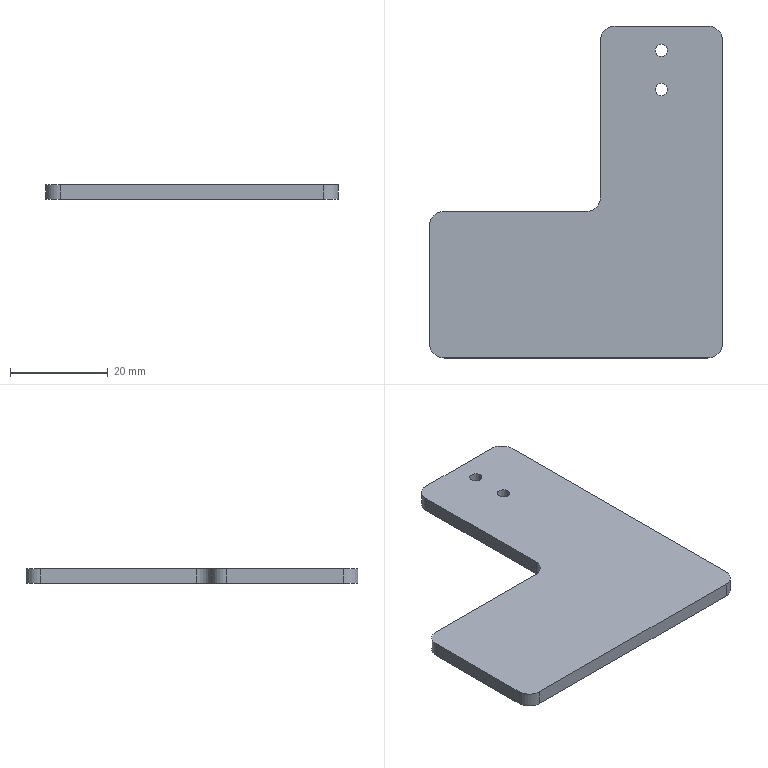Part | STEP file | 001-006-Pre-insertion mechanism drag chain mounting plate | 1 solid | 18 faces | box 60 x 68 x 3 mm | volume 8197 mm3 | cylinder 10 | plane 8 | commonest cylinder face diameters 6 x6 2.5 x4
STEP:
#1=CARTESIAN_POINT('',(0.,0.,0.));
#2=DIRECTION('',(0.,0.,1.));
#3=DIRECTION('',(1.,0.,0.));
#4=AXIS2_PLACEMENT_3D('',#1,#2,#3);
#5=CARTESIAN_POINT('',(18.75,29.,-3.));
#6=VERTEX_POINT('',#5);
#7=CARTESIAN_POINT('',(18.75,29.,0.));
#8=VERTEX_POINT('',#7);
#9=CARTESIAN_POINT('',(18.75,29.,0.));
#10=DIRECTION('',(0.,0.,1.));
#11=VECTOR('',#10,1.);
#12=LINE('',#9,#11);
#13=CARTESIAN_POINT('',(17.5,29.,0.));
#14=DIRECTION('',(0.,0.,1.));
#15=DIRECTION('',(1.,0.,0.));
#16=AXIS2_PLACEMENT_3D('',#13,#14,#15);
#17=CYLINDRICAL_SURFACE('',#16,1.25);
#18=CARTESIAN_POINT('',(6.283,0.));
#19=DIRECTION('',(0.,1.));
#20=VECTOR('',#19,1.);
#21=LINE('',#18,#20);
#22=(GEOMETRIC_REPRESENTATION_CONTEXT(2)PARAMETRIC_REPRESENTATION_CONTEXT()REPRESENTATION_CONTEXT('',''));
#23=DEFINITIONAL_REPRESENTATION('',(#21),#22);
#24=PCURVE('',#17,#23);
#25=CARTESIAN_POINT('',(17.5,29.,0.));
#26=DIRECTION('',(0.,0.,1.));
#27=DIRECTION('',(1.,0.,0.));
#28=AXIS2_PLACEMENT_3D('',#25,#26,#27);
#29=CYLINDRICAL_SURFACE('',#28,1.25);
#30=CARTESIAN_POINT('',(0.,0.));
#31=DIRECTION('',(0.,1.));
#32=VECTOR('',#31,1.);
#33=LINE('',#30,#32);
#34=(GEOMETRIC_REPRESENTATION_CONTEXT(2)PARAMETRIC_REPRESENTATION_CONTEXT()REPRESENTATION_CONTEXT('',''));
#35=DEFINITIONAL_REPRESENTATION('',(#33),#34);
#36=PCURVE('',#29,#35);
#37=SURFACE_CURVE('',#12,(#24,#36),.PCURVE_S1.);
#38=EDGE_CURVE('',#6,#8,#37,.T.);
#39=ORIENTED_EDGE('',*,*,#38,.T.);
#40=CARTESIAN_POINT('',(16.25,29.,0.));
#41=VERTEX_POINT('',#40);
#42=CARTESIAN_POINT('',(17.5,29.,0.));
#43=DIRECTION('',(0.,0.,1.));
#44=DIRECTION('',(1.,0.,0.));
#45=AXIS2_PLACEMENT_3D('',#42,#43,#44);
#46=CIRCLE('',#45,1.25);
#47=CARTESIAN_POINT('',(0.,0.));
#48=DIRECTION('',(1.,0.));
#49=VECTOR('',#48,1.);
#50=LINE('',#47,#49);
#51=(GEOMETRIC_REPRESENTATION_CONTEXT(2)PARAMETRIC_REPRESENTATION_CONTEXT()REPRESENTATION_CONTEXT('',''));
#52=DEFINITIONAL_REPRESENTATION('',(#50),#51);
#53=PCURVE('',#17,#52);
#54=CARTESIAN_POINT('',(0.,0.,0.));
#55=DIRECTION('',(0.,0.,-1.));
#56=DIRECTION('',(-1.,0.,0.));
#57=AXIS2_PLACEMENT_3D('',#54,#55,#56);
#58=PLANE('',#57);
#59=CARTESIAN_POINT('',(-18.75,29.));
#60=CARTESIAN_POINT('',(-18.75,31.165));
#61=CARTESIAN_POINT('',(-16.875,30.083));
#62=CARTESIAN_POINT('',(-15.,29.));
#63=CARTESIAN_POINT('',(-16.875,27.917));
#64=CARTESIAN_POINT('',(-18.75,26.835));
#65=CARTESIAN_POINT('',(-18.75,29.));
#66=(BOUNDED_CURVE()B_SPLINE_CURVE(2,(#59,#60,#61,#62,#63,#64,#65),.UNSPECIFIED.,.T.,.F.)B_SPLINE_CURVE_WITH_KNOTS((1,2,2,2,2,1),(-2.094,0.,2.094,4.189,6.283,8.378),.UNSPECIFIED.)CURVE()GEOMETRIC_REPRESENTATION_ITEM()RATIONAL_B_SPLINE_CURVE((1.,0.5,1.,0.5,1.,0.5,1.))REPRESENTATION_ITEM(''));
#67=(GEOMETRIC_REPRESENTATION_CONTEXT(2)PARAMETRIC_REPRESENTATION_CONTEXT()REPRESENTATION_CONTEXT('',''));
#68=DEFINITIONAL_REPRESENTATION('',(#66),#67);
#69=PCURVE('',#58,#68);
#70=SURFACE_CURVE('',#46,(#53,#69),.PCURVE_S1.);
#71=EDGE_CURVE('',#41,#8,#70,.T.);
#72=ORIENTED_EDGE('',*,*,#71,.F.);
#73=CARTESIAN_POINT('',(16.25,29.,-3.));
#74=VERTEX_POINT('',#73);
#75=CARTESIAN_POINT('',(16.25,29.,0.));
#76=DIRECTION('',(0.,0.,1.));
#77=VECTOR('',#76,1.);
#78=LINE('',#75,#77);
#79=CARTESIAN_POINT('',(3.142,0.));
#80=DIRECTION('',(0.,1.));
#81=VECTOR('',#80,1.);
#82=LINE('',#79,#81);
#83=(GEOMETRIC_REPRESENTATION_CONTEXT(2)PARAMETRIC_REPRESENTATION_CONTEXT()REPRESENTATION_CONTEXT('',''));
#84=DEFINITIONAL_REPRESENTATION('',(#82),#83);
#85=PCURVE('',#17,#84);
#86=CARTESIAN_POINT('',(3.142,0.));
#87=DIRECTION('',(0.,1.));
#88=VECTOR('',#87,1.);
#89=LINE('',#86,#88);
#90=(GEOMETRIC_REPRESENTATION_CONTEXT(2)PARAMETRIC_REPRESENTATION_CONTEXT()REPRESENTATION_CONTEXT('',''));
#91=DEFINITIONAL_REPRESENTATION('',(#89),#90);
#92=PCURVE('',#29,#91);
#93=SURFACE_CURVE('',#78,(#85,#92),.PCURVE_S1.);
#94=EDGE_CURVE('',#74,#41,#93,.T.);
#95=ORIENTED_EDGE('',*,*,#94,.F.);
#96=CARTESIAN_POINT('',(17.5,29.,-3.));
#97=DIRECTION('',(0.,0.,1.));
#98=DIRECTION('',(1.,0.,0.));
#99=AXIS2_PLACEMENT_3D('',#96,#97,#98);
#100=CIRCLE('',#99,1.25);
#101=CARTESIAN_POINT('',(0.,-3.));
#102=DIRECTION('',(1.,0.));
#103=VECTOR('',#102,1.);
#104=LINE('',#101,#103);
#105=(GEOMETRIC_REPRESENTATION_CONTEXT(2)PARAMETRIC_REPRESENTATION_CONTEXT()REPRESENTATION_CONTEXT('',''));
#106=DEFINITIONAL_REPRESENTATION('',(#104),#105);
#107=PCURVE('',#17,#106);
#108=CARTESIAN_POINT('',(0.,0.,-3.));
#109=DIRECTION('',(0.,0.,-1.));
#110=DIRECTION('',(-1.,0.,0.));
#111=AXIS2_PLACEMENT_3D('',#108,#109,#110);
#112=PLANE('',#111);
#113=CARTESIAN_POINT('',(-18.75,29.));
#114=CARTESIAN_POINT('',(-18.75,31.165));
#115=CARTESIAN_POINT('',(-16.875,30.083));
#116=CARTESIAN_POINT('',(-15.,29.));
#117=CARTESIAN_POINT('',(-16.875,27.917));
#118=CARTESIAN_POINT('',(-18.75,26.835));
#119=CARTESIAN_POINT('',(-18.75,29.));
#120=(BOUNDED_CURVE()B_SPLINE_CURVE(2,(#113,#114,#115,#116,#117,#118,#119),.UNSPECIFIED.,.T.,.F.)B_SPLINE_CURVE_WITH_KNOTS((1,2,2,2,2,1),(-2.094,0.,2.094,4.189,6.283,8.378),.UNSPECIFIED.)CURVE()GEOMETRIC_REPRESENTATION_ITEM()RATIONAL_B_SPLINE_CURVE((1.,0.5,1.,0.5,1.,0.5,1.))REPRESENTATION_ITEM(''));
#121=(GEOMETRIC_REPRESENTATION_CONTEXT(2)PARAMETRIC_REPRESENTATION_CONTEXT()REPRESENTATION_CONTEXT('',''));
#122=DEFINITIONAL_REPRESENTATION('',(#120),#121);
#123=PCURVE('',#112,#122);
#124=SURFACE_CURVE('',#100,(#107,#123),.PCURVE_S1.);
#125=EDGE_CURVE('',#74,#6,#124,.T.);
#126=ORIENTED_EDGE('',*,*,#125,.T.);
#127=EDGE_LOOP('',(#39,#72,#95,#126));
#128=FACE_BOUND('',#127,.F.);
#129=ADVANCED_FACE('',(#128),#17,.F.);
#130=CARTESIAN_POINT('',(18.75,21.,-3.));
#131=VERTEX_POINT('',#130);
#132=CARTESIAN_POINT('',(18.75,21.,0.));
#133=VERTEX_POINT('',#132);
#134=CARTESIAN_POINT('',(18.75,21.,0.));
#135=DIRECTION('',(0.,0.,1.));
#136=VECTOR('',#135,1.);
#137=LINE('',#134,#136);
#138=CARTESIAN_POINT('',(17.5,21.,0.));
#139=DIRECTION('',(0.,0.,1.));
#140=DIRECTION('',(1.,0.,0.));
#141=AXIS2_PLACEMENT_3D('',#138,#139,#140);
#142=CYLINDRICAL_SURFACE('',#141,1.25);
#143=CARTESIAN_POINT('',(6.283,0.));
#144=DIRECTION('',(0.,1.));
#145=VECTOR('',#144,1.);
#146=LINE('',#143,#145);
#147=(GEOMETRIC_REPRESENTATION_CONTEXT(2)PARAMETRIC_REPRESENTATION_CONTEXT()REPRESENTATION_CONTEXT('',''));
#148=DEFINITIONAL_REPRESENTATION('',(#146),#147);
#149=PCURVE('',#142,#148);
#150=CARTESIAN_POINT('',(17.5,21.,0.));
#151=DIRECTION('',(0.,0.,1.));
#152=DIRECTION('',(1.,0.,0.));
#153=AXIS2_PLACEMENT_3D('',#150,#151,#152);
#154=CYLINDRICAL_SURFACE('',#153,1.25);
#155=CARTESIAN_POINT('',(0.,0.));
#156=DIRECTION('',(0.,1.));
#157=VECTOR('',#156,1.);
#158=LINE('',#155,#157);
#159=(GEOMETRIC_REPRESENTATION_CONTEXT(2)PARAMETRIC_REPRESENTATION_CONTEXT()REPRESENTATION_CONTEXT('',''));
#160=DEFINITIONAL_REPRESENTATION('',(#158),#159);
#161=PCURVE('',#154,#160);
#162=SURFACE_CURVE('',#137,(#149,#161),.PCURVE_S1.);
#163=EDGE_CURVE('',#131,#133,#162,.T.);
#164=ORIENTED_EDGE('',*,*,#163,.T.);
#165=CARTESIAN_POINT('',(16.25,21.,0.));
#166=VERTEX_POINT('',#165);
#167=CARTESIAN_POINT('',(17.5,21.,0.));
#168=DIRECTION('',(0.,0.,1.));
#169=DIRECTION('',(1.,0.,0.));
#170=AXIS2_PLACEMENT_3D('',#167,#168,#169);
#171=CIRCLE('',#170,1.25);
#172=CARTESIAN_POINT('',(0.,0.));
#173=DIRECTION('',(1.,0.));
#174=VECTOR('',#173,1.);
#175=LINE('',#172,#174);
#176=(GEOMETRIC_REPRESENTATION_CONTEXT(2)PARAMETRIC_REPRESENTATION_CONTEXT()REPRESENTATION_CONTEXT('',''));
#177=DEFINITIONAL_REPRESENTATION('',(#175),#176);
#178=PCURVE('',#142,#177);
#179=CARTESIAN_POINT('',(-18.75,21.));
#180=CARTESIAN_POINT('',(-18.75,23.165));
#181=CARTESIAN_POINT('',(-16.875,22.083));
#182=CARTESIAN_POINT('',(-15.,21.));
#183=CARTESIAN_POINT('',(-16.875,19.917));
#184=CARTESIAN_POINT('',(-18.75,18.835));
#185=CARTESIAN_POINT('',(-18.75,21.));
#186=(BOUNDED_CURVE()B_SPLINE_CURVE(2,(#179,#180,#181,#182,#183,#184,#185),.UNSPECIFIED.,.T.,.F.)B_SPLINE_CURVE_WITH_KNOTS((1,2,2,2,2,1),(-2.094,0.,2.094,4.189,6.283,8.378),.UNSPECIFIED.)CURVE()GEOMETRIC_REPRESENTATION_ITEM()RATIONAL_B_SPLINE_CURVE((1.,0.5,1.,0.5,1.,0.5,1.))REPRESENTATION_ITEM(''));
#187=(GEOMETRIC_REPRESENTATION_CONTEXT(2)PARAMETRIC_REPRESENTATION_CONTEXT()REPRESENTATION_CONTEXT('',''));
#188=DEFINITIONAL_REPRESENTATION('',(#186),#187);
#189=PCURVE('',#58,#188);
#190=SURFACE_CURVE('',#171,(#178,#189),.PCURVE_S1.);
#191=EDGE_CURVE('',#166,#133,#190,.T.);
#192=ORIENTED_EDGE('',*,*,#191,.F.);
#193=CARTESIAN_POINT('',(16.25,21.,-3.));
#194=VERTEX_POINT('',#193);
#195=CARTESIAN_POINT('',(16.25,21.,0.));
#196=DIRECTION('',(0.,0.,1.));
#197=VECTOR('',#196,1.);
#198=LINE('',#195,#197);
#199=CARTESIAN_POINT('',(3.142,0.));
#200=DIRECTION('',(0.,1.));
#201=VECTOR('',#200,1.);
#202=LINE('',#199,#201);
#203=(GEOMETRIC_REPRESENTATION_CONTEXT(2)PARAMETRIC_REPRESENTATION_CONTEXT()REPRESENTATION_CONTEXT('',''));
#204=DEFINITIONAL_REPRESENTATION('',(#202),#203);
#205=PCURVE('',#142,#204);
#206=CARTESIAN_POINT('',(3.142,0.));
#207=DIRECTION('',(0.,1.));
#208=VECTOR('',#207,1.);
#209=LINE('',#206,#208);
#210=(GEOMETRIC_REPRESENTATION_CONTEXT(2)PARAMETRIC_REPRESENTATION_CONTEXT()REPRESENTATION_CONTEXT('',''));
#211=DEFINITIONAL_REPRESENTATION('',(#209),#210);
#212=PCURVE('',#154,#211);
#213=SURFACE_CURVE('',#198,(#205,#212),.PCURVE_S1.);
#214=EDGE_CURVE('',#194,#166,#213,.T.);
#215=ORIENTED_EDGE('',*,*,#214,.F.);
#216=CARTESIAN_POINT('',(17.5,21.,-3.));
#217=DIRECTION('',(0.,0.,1.));
#218=DIRECTION('',(1.,0.,0.));
#219=AXIS2_PLACEMENT_3D('',#216,#217,#218);
#220=CIRCLE('',#219,1.25);
#221=CARTESIAN_POINT('',(0.,-3.));
#222=DIRECTION('',(1.,0.));
#223=VECTOR('',#222,1.);
#224=LINE('',#221,#223);
#225=(GEOMETRIC_REPRESENTATION_CONTEXT(2)PARAMETRIC_REPRESENTATION_CONTEXT()REPRESENTATION_CONTEXT('',''));
#226=DEFINITIONAL_REPRESENTATION('',(#224),#225);
#227=PCURVE('',#142,#226);
#228=CARTESIAN_POINT('',(-18.75,21.));
#229=CARTESIAN_POINT('',(-18.75,23.165));
#230=CARTESIAN_POINT('',(-16.875,22.083));
#231=CARTESIAN_POINT('',(-15.,21.));
#232=CARTESIAN_POINT('',(-16.875,19.917));
#233=CARTESIAN_POINT('',(-18.75,18.835));
#234=CARTESIAN_POINT('',(-18.75,21.));
#235=(BOUNDED_CURVE()B_SPLINE_CURVE(2,(#228,#229,#230,#231,#232,#233,#234),.UNSPECIFIED.,.T.,.F.)B_SPLINE_CURVE_WITH_KNOTS((1,2,2,2,2,1),(-2.094,0.,2.094,4.189,6.283,8.378),.UNSPECIFIED.)CURVE()GEOMETRIC_REPRESENTATION_ITEM()RATIONAL_B_SPLINE_CURVE((1.,0.5,1.,0.5,1.,0.5,1.))REPRESENTATION_ITEM(''));
#236=(GEOMETRIC_REPRESENTATION_CONTEXT(2)PARAMETRIC_REPRESENTATION_CONTEXT()REPRESENTATION_CONTEXT('',''));
#237=DEFINITIONAL_REPRESENTATION('',(#235),#236);
#238=PCURVE('',#112,#237);
#239=SURFACE_CURVE('',#220,(#227,#238),.PCURVE_S1.);
#240=EDGE_CURVE('',#194,#131,#239,.T.);
#241=ORIENTED_EDGE('',*,*,#240,.T.);
#242=EDGE_LOOP('',(#164,#192,#215,#241));
#243=FACE_BOUND('',#242,.F.);
#244=ADVANCED_FACE('',(#243),#142,.F.);
#245=CARTESIAN_POINT('',(-30.,-7.,-3.));
#246=VERTEX_POINT('',#245);
#247=CARTESIAN_POINT('',(-30.,-31.,-3.));
#248=VERTEX_POINT('',#247);
#249=CARTESIAN_POINT('',(-30.,-34.,-3.));
#250=DIRECTION('',(0.,-1.,0.));
#251=VECTOR('',#250,1.);
#252=LINE('',#249,#251);
#253=CARTESIAN_POINT('',(30.,-34.));
#254=DIRECTION('',(0.,-1.));
#255=VECTOR('',#254,1.);
#256=LINE('',#253,#255);
#257=(GEOMETRIC_REPRESENTATION_CONTEXT(2)PARAMETRIC_REPRESENTATION_CONTEXT()REPRESENTATION_CONTEXT('',''));
#258=DEFINITIONAL_REPRESENTATION('',(#256),#257);
#259=PCURVE('',#112,#258);
#260=CARTESIAN_POINT('',(-30.,-34.,-3.));
#261=DIRECTION('',(-1.,0.,0.));
#262=DIRECTION('',(0.,0.,1.));
#263=AXIS2_PLACEMENT_3D('',#260,#261,#262);
#264=PLANE('',#263);
#265=CARTESIAN_POINT('',(0.,0.));
#266=DIRECTION('',(0.,-1.));
#267=VECTOR('',#266,1.);
#268=LINE('',#265,#267);
#269=(GEOMETRIC_REPRESENTATION_CONTEXT(2)PARAMETRIC_REPRESENTATION_CONTEXT()REPRESENTATION_CONTEXT('',''));
#270=DEFINITIONAL_REPRESENTATION('',(#268),#269);
#271=PCURVE('',#264,#270);
#272=SURFACE_CURVE('',#252,(#259,#271),.PCURVE_S1.);
#273=EDGE_CURVE('',#246,#248,#272,.T.);
#274=ORIENTED_EDGE('',*,*,#273,.F.);
#275=CARTESIAN_POINT('',(-27.,-4.,-3.));
#276=VERTEX_POINT('',#275);
#277=CARTESIAN_POINT('',(-27.,-7.,-3.));
#278=DIRECTION('',(0.,0.,-1.));
#279=DIRECTION('',(-1.,0.,0.));
#280=AXIS2_PLACEMENT_3D('',#277,#278,#279);
#281=CIRCLE('',#280,3.);
#282=CARTESIAN_POINT('',(27.,-7.));
#283=DIRECTION('',(1.,0.));
#284=AXIS2_PLACEMENT_2D('',#282,#283);
#285=CIRCLE('',#284,3.);
#286=(GEOMETRIC_REPRESENTATION_CONTEXT(2)PARAMETRIC_REPRESENTATION_CONTEXT()REPRESENTATION_CONTEXT('',''));
#287=DEFINITIONAL_REPRESENTATION('',(#285),#286);
#288=PCURVE('',#112,#287);
#289=CARTESIAN_POINT('',(-27.,-7.,-10.));
#290=DIRECTION('',(0.,0.,-1.));
#291=DIRECTION('',(-1.,0.,0.));
#292=AXIS2_PLACEMENT_3D('',#289,#290,#291);
#293=CYLINDRICAL_SURFACE('',#292,3.);
#294=CARTESIAN_POINT('',(0.,-7.));
#295=DIRECTION('',(1.,0.));
#296=VECTOR('',#295,1.);
#297=LINE('',#294,#296);
#298=(GEOMETRIC_REPRESENTATION_CONTEXT(2)PARAMETRIC_REPRESENTATION_CONTEXT()REPRESENTATION_CONTEXT('',''));
#299=DEFINITIONAL_REPRESENTATION('',(#297),#298);
#300=PCURVE('',#293,#299);
#301=SURFACE_CURVE('',#281,(#288,#300),.PCURVE_S1.);
#302=EDGE_CURVE('',#246,#276,#301,.T.);
#303=ORIENTED_EDGE('',*,*,#302,.T.);
#304=CARTESIAN_POINT('',(2.,-4.,-3.));
#305=VERTEX_POINT('',#304);
#306=CARTESIAN_POINT('',(0.,-4.,-3.));
#307=DIRECTION('',(-1.,0.,0.));
#308=VECTOR('',#307,1.);
#309=LINE('',#306,#308);
#310=CARTESIAN_POINT('',(0.,-4.));
#311=DIRECTION('',(1.,0.));
#312=VECTOR('',#311,1.);
#313=LINE('',#310,#312);
#314=(GEOMETRIC_REPRESENTATION_CONTEXT(2)PARAMETRIC_REPRESENTATION_CONTEXT()REPRESENTATION_CONTEXT('',''));
#315=DEFINITIONAL_REPRESENTATION('',(#313),#314);
#316=PCURVE('',#112,#315);
#317=CARTESIAN_POINT('',(-30.,-4.,-10.));
#318=DIRECTION('',(0.,-1.,0.));
#319=DIRECTION('',(0.,0.,-1.));
#320=AXIS2_PLACEMENT_3D('',#317,#318,#319);
#321=PLANE('',#320);
#322=CARTESIAN_POINT('',(-7.,30.));
#323=DIRECTION('',(0.,-1.));
#324=VECTOR('',#323,1.);
#325=LINE('',#322,#324);
#326=(GEOMETRIC_REPRESENTATION_CONTEXT(2)PARAMETRIC_REPRESENTATION_CONTEXT()REPRESENTATION_CONTEXT('',''));
#327=DEFINITIONAL_REPRESENTATION('',(#325),#326);
#328=PCURVE('',#321,#327);
#329=SURFACE_CURVE('',#309,(#316,#328),.PCURVE_S1.);
#330=EDGE_CURVE('',#305,#276,#329,.T.);
#331=ORIENTED_EDGE('',*,*,#330,.F.);
#332=CARTESIAN_POINT('',(5.,-1.,-3.));
#333=VERTEX_POINT('',#332);
#334=CARTESIAN_POINT('',(2.,-1.,-3.));
#335=DIRECTION('',(0.,0.,1.));
#336=DIRECTION('',(-1.,0.,0.));
#337=AXIS2_PLACEMENT_3D('',#334,#335,#336);
#338=CIRCLE('',#337,3.);
#339=CARTESIAN_POINT('',(1.,-1.));
#340=CARTESIAN_POINT('',(1.,-6.196));
#341=CARTESIAN_POINT('',(-3.5,-3.598));
#342=CARTESIAN_POINT('',(-8.,-1.));
#343=CARTESIAN_POINT('',(-3.5,1.598));
#344=CARTESIAN_POINT('',(1.,4.196));
#345=CARTESIAN_POINT('',(1.,-1.));
#346=(BOUNDED_CURVE()B_SPLINE_CURVE(2,(#339,#340,#341,#342,#343,#344,#345),.UNSPECIFIED.,.T.,.F.)B_SPLINE_CURVE_WITH_KNOTS((1,2,2,2,2,1),(-2.094,0.,2.094,4.189,6.283,8.378),.UNSPECIFIED.)CURVE()GEOMETRIC_REPRESENTATION_ITEM()RATIONAL_B_SPLINE_CURVE((1.,0.5,1.,0.5,1.,0.5,1.))REPRESENTATION_ITEM(''));
#347=(GEOMETRIC_REPRESENTATION_CONTEXT(2)PARAMETRIC_REPRESENTATION_CONTEXT()REPRESENTATION_CONTEXT('',''));
#348=DEFINITIONAL_REPRESENTATION('',(#346),#347);
#349=PCURVE('',#112,#348);
#350=CARTESIAN_POINT('',(2.,-1.,-10.));
#351=DIRECTION('',(0.,0.,-1.));
#352=DIRECTION('',(-1.,0.,0.));
#353=AXIS2_PLACEMENT_3D('',#350,#351,#352);
#354=CYLINDRICAL_SURFACE('',#353,3.);
#355=CARTESIAN_POINT('',(6.283,-7.));
#356=DIRECTION('',(-1.,0.));
#357=VECTOR('',#356,1.);
#358=LINE('',#355,#357);
#359=(GEOMETRIC_REPRESENTATION_CONTEXT(2)PARAMETRIC_REPRESENTATION_CONTEXT()REPRESENTATION_CONTEXT('',''));
#360=DEFINITIONAL_REPRESENTATION('',(#358),#359);
#361=PCURVE('',#354,#360);
#362=SURFACE_CURVE('',#338,(#349,#361),.PCURVE_S1.);
#363=EDGE_CURVE('',#305,#333,#362,.T.);
#364=ORIENTED_EDGE('',*,*,#363,.T.);
#365=CARTESIAN_POINT('',(5.,31.,-3.));
#366=VERTEX_POINT('',#365);
#367=CARTESIAN_POINT('',(5.,0.,-3.));
#368=DIRECTION('',(0.,-1.,0.));
#369=VECTOR('',#368,1.);
#370=LINE('',#367,#369);
#371=CARTESIAN_POINT('',(-5.,0.));
#372=DIRECTION('',(0.,-1.));
#373=VECTOR('',#372,1.);
#374=LINE('',#371,#373);
#375=(GEOMETRIC_REPRESENTATION_CONTEXT(2)PARAMETRIC_REPRESENTATION_CONTEXT()REPRESENTATION_CONTEXT('',''));
#376=DEFINITIONAL_REPRESENTATION('',(#374),#375);
#377=PCURVE('',#112,#376);
#378=CARTESIAN_POINT('',(5.,34.,-10.));
#379=DIRECTION('',(1.,0.,0.));
#380=DIRECTION('',(0.,1.,0.));
#381=AXIS2_PLACEMENT_3D('',#378,#379,#380);
#382=PLANE('',#381);
#383=CARTESIAN_POINT('',(-34.,7.));
#384=DIRECTION('',(-1.,0.));
#385=VECTOR('',#384,1.);
#386=LINE('',#383,#385);
#387=(GEOMETRIC_REPRESENTATION_CONTEXT(2)PARAMETRIC_REPRESENTATION_CONTEXT()REPRESENTATION_CONTEXT('',''));
#388=DEFINITIONAL_REPRESENTATION('',(#386),#387);
#389=PCURVE('',#382,#388);
#390=SURFACE_CURVE('',#370,(#377,#389),.PCURVE_S1.);
#391=EDGE_CURVE('',#366,#333,#390,.T.);
#392=ORIENTED_EDGE('',*,*,#391,.F.);
#393=CARTESIAN_POINT('',(8.,34.,-3.));
#394=VERTEX_POINT('',#393);
#395=CARTESIAN_POINT('',(8.,31.,-3.));
#396=DIRECTION('',(0.,0.,-1.));
#397=DIRECTION('',(-1.,0.,0.));
#398=AXIS2_PLACEMENT_3D('',#395,#396,#397);
#399=CIRCLE('',#398,3.);
#400=CARTESIAN_POINT('',(-8.,31.));
#401=DIRECTION('',(1.,0.));
#402=AXIS2_PLACEMENT_2D('',#400,#401);
#403=CIRCLE('',#402,3.);
#404=(GEOMETRIC_REPRESENTATION_CONTEXT(2)PARAMETRIC_REPRESENTATION_CONTEXT()REPRESENTATION_CONTEXT('',''));
#405=DEFINITIONAL_REPRESENTATION('',(#403),#404);
#406=PCURVE('',#112,#405);
#407=CARTESIAN_POINT('',(8.,31.,-3.));
#408=DIRECTION('',(0.,0.,-1.));
#409=DIRECTION('',(-1.,0.,0.));
#410=AXIS2_PLACEMENT_3D('',#407,#408,#409);
#411=CYLINDRICAL_SURFACE('',#410,3.);
#412=CARTESIAN_POINT('',(0.,0.));
#413=DIRECTION('',(1.,0.));
#414=VECTOR('',#413,1.);
#415=LINE('',#412,#414);
#416=(GEOMETRIC_REPRESENTATION_CONTEXT(2)PARAMETRIC_REPRESENTATION_CONTEXT()REPRESENTATION_CONTEXT('',''));
#417=DEFINITIONAL_REPRESENTATION('',(#415),#416);
#418=PCURVE('',#411,#417);
#419=SURFACE_CURVE('',#399,(#406,#418),.PCURVE_S1.);
#420=EDGE_CURVE('',#366,#394,#419,.T.);
#421=ORIENTED_EDGE('',*,*,#420,.T.);
#422=CARTESIAN_POINT('',(27.,34.,-3.));
#423=VERTEX_POINT('',#422);
#424=CARTESIAN_POINT('',(-30.,34.,-3.));
#425=DIRECTION('',(-1.,0.,0.));
#426=VECTOR('',#425,1.);
#427=LINE('',#424,#426);
#428=CARTESIAN_POINT('',(30.,34.));
#429=DIRECTION('',(1.,0.));
#430=VECTOR('',#429,1.);
#431=LINE('',#428,#430);
#432=(GEOMETRIC_REPRESENTATION_CONTEXT(2)PARAMETRIC_REPRESENTATION_CONTEXT()REPRESENTATION_CONTEXT('',''));
#433=DEFINITIONAL_REPRESENTATION('',(#431),#432);
#434=PCURVE('',#112,#433);
#435=CARTESIAN_POINT('',(-30.,34.,-3.));
#436=DIRECTION('',(0.,1.,0.));
#437=DIRECTION('',(-1.,0.,0.));
#438=AXIS2_PLACEMENT_3D('',#435,#436,#437);
#439=PLANE('',#438);
#440=CARTESIAN_POINT('',(0.,0.));
#441=DIRECTION('',(1.,0.));
#442=VECTOR('',#441,1.);
#443=LINE('',#440,#442);
#444=(GEOMETRIC_REPRESENTATION_CONTEXT(2)PARAMETRIC_REPRESENTATION_CONTEXT()REPRESENTATION_CONTEXT('',''));
#445=DEFINITIONAL_REPRESENTATION('',(#443),#444);
#446=PCURVE('',#439,#445);
#447=SURFACE_CURVE('',#427,(#434,#446),.PCURVE_S1.);
#448=EDGE_CURVE('',#423,#394,#447,.T.);
#449=ORIENTED_EDGE('',*,*,#448,.F.);
#450=CARTESIAN_POINT('',(30.,31.,-3.));
#451=VERTEX_POINT('',#450);
#452=CARTESIAN_POINT('',(27.,31.,-3.));
#453=DIRECTION('',(0.,0.,-1.));
#454=DIRECTION('',(-1.,0.,0.));
#455=AXIS2_PLACEMENT_3D('',#452,#453,#454);
#456=CIRCLE('',#455,3.);
#457=CARTESIAN_POINT('',(-27.,31.));
#458=DIRECTION('',(1.,0.));
#459=AXIS2_PLACEMENT_2D('',#457,#458);
#460=CIRCLE('',#459,3.);
#461=(GEOMETRIC_REPRESENTATION_CONTEXT(2)PARAMETRIC_REPRESENTATION_CONTEXT()REPRESENTATION_CONTEXT('',''));
#462=DEFINITIONAL_REPRESENTATION('',(#460),#461);
#463=PCURVE('',#112,#462);
#464=CARTESIAN_POINT('',(27.,31.,-3.));
#465=DIRECTION('',(0.,0.,1.));
#466=DIRECTION('',(1.,0.,0.));
#467=AXIS2_PLACEMENT_3D('',#464,#465,#466);
#468=CYLINDRICAL_SURFACE('',#467,3.);
#469=CARTESIAN_POINT('',(3.142,0.));
#470=DIRECTION('',(-1.,0.));
#471=VECTOR('',#470,1.);
#472=LINE('',#469,#471);
#473=(GEOMETRIC_REPRESENTATION_CONTEXT(2)PARAMETRIC_REPRESENTATION_CONTEXT()REPRESENTATION_CONTEXT('',''));
#474=DEFINITIONAL_REPRESENTATION('',(#472),#473);
#475=PCURVE('',#468,#474);
#476=SURFACE_CURVE('',#456,(#463,#475),.PCURVE_S1.);
#477=EDGE_CURVE('',#423,#451,#476,.T.);
#478=ORIENTED_EDGE('',*,*,#477,.T.);
#479=CARTESIAN_POINT('',(30.,-31.,-3.));
#480=VERTEX_POINT('',#479);
#481=CARTESIAN_POINT('',(30.,-34.,-3.));
#482=DIRECTION('',(0.,1.,0.));
#483=VECTOR('',#482,1.);
#484=LINE('',#481,#483);
#485=CARTESIAN_POINT('',(-30.,-34.));
#486=DIRECTION('',(0.,1.));
#487=VECTOR('',#486,1.);
#488=LINE('',#485,#487);
#489=(GEOMETRIC_REPRESENTATION_CONTEXT(2)PARAMETRIC_REPRESENTATION_CONTEXT()REPRESENTATION_CONTEXT('',''));
#490=DEFINITIONAL_REPRESENTATION('',(#488),#489);
#491=PCURVE('',#112,#490);
#492=CARTESIAN_POINT('',(30.,-34.,-3.));
#493=DIRECTION('',(1.,0.,0.));
#494=DIRECTION('',(0.,1.,0.));
#495=AXIS2_PLACEMENT_3D('',#492,#493,#494);
#496=PLANE('',#495);
#497=CARTESIAN_POINT('',(0.,0.));
#498=DIRECTION('',(1.,0.));
#499=VECTOR('',#498,1.);
#500=LINE('',#497,#499);
#501=(GEOMETRIC_REPRESENTATION_CONTEXT(2)PARAMETRIC_REPRESENTATION_CONTEXT()REPRESENTATION_CONTEXT('',''));
#502=DEFINITIONAL_REPRESENTATION('',(#500),#501);
#503=PCURVE('',#496,#502);
#504=SURFACE_CURVE('',#484,(#491,#503),.PCURVE_S1.);
#505=EDGE_CURVE('',#480,#451,#504,.T.);
#506=ORIENTED_EDGE('',*,*,#505,.F.);
#507=CARTESIAN_POINT('',(27.,-34.,-3.));
#508=VERTEX_POINT('',#507);
#509=CARTESIAN_POINT('',(27.,-31.,-3.));
#510=DIRECTION('',(0.,0.,-1.));
#511=DIRECTION('',(-1.,0.,0.));
#512=AXIS2_PLACEMENT_3D('',#509,#510,#511);
#513=CIRCLE('',#512,3.);
#514=CARTESIAN_POINT('',(-27.,-31.));
#515=DIRECTION('',(1.,0.));
#516=AXIS2_PLACEMENT_2D('',#514,#515);
#517=CIRCLE('',#516,3.);
#518=(GEOMETRIC_REPRESENTATION_CONTEXT(2)PARAMETRIC_REPRESENTATION_CONTEXT()REPRESENTATION_CONTEXT('',''));
#519=DEFINITIONAL_REPRESENTATION('',(#517),#518);
#520=PCURVE('',#112,#519);
#521=CARTESIAN_POINT('',(27.,-31.,-3.));
#522=DIRECTION('',(0.,0.,1.));
#523=DIRECTION('',(1.,0.,0.));
#524=AXIS2_PLACEMENT_3D('',#521,#522,#523);
#525=CYLINDRICAL_SURFACE('',#524,3.);
#526=CARTESIAN_POINT('',(9.425,0.));
#527=DIRECTION('',(-1.,0.));
#528=VECTOR('',#527,1.);
#529=LINE('',#526,#528);
#530=(GEOMETRIC_REPRESENTATION_CONTEXT(2)PARAMETRIC_REPRESENTATION_CONTEXT()REPRESENTATION_CONTEXT('',''));
#531=DEFINITIONAL_REPRESENTATION('',(#529),#530);
#532=PCURVE('',#525,#531);
#533=SURFACE_CURVE('',#513,(#520,#532),.PCURVE_S1.);
#534=EDGE_CURVE('',#480,#508,#533,.T.);
#535=ORIENTED_EDGE('',*,*,#534,.T.);
#536=CARTESIAN_POINT('',(-27.,-34.,-3.));
#537=VERTEX_POINT('',#536);
#538=CARTESIAN_POINT('',(-30.,-34.,-3.));
#539=DIRECTION('',(1.,0.,0.));
#540=VECTOR('',#539,1.);
#541=LINE('',#538,#540);
#542=CARTESIAN_POINT('',(30.,-34.));
#543=DIRECTION('',(-1.,0.));
#544=VECTOR('',#543,1.);
#545=LINE('',#542,#544);
#546=(GEOMETRIC_REPRESENTATION_CONTEXT(2)PARAMETRIC_REPRESENTATION_CONTEXT()REPRESENTATION_CONTEXT('',''));
#547=DEFINITIONAL_REPRESENTATION('',(#545),#546);
#548=PCURVE('',#112,#547);
#549=CARTESIAN_POINT('',(-30.,-34.,-3.));
#550=DIRECTION('',(0.,-1.,0.));
#551=DIRECTION('',(1.,0.,0.));
#552=AXIS2_PLACEMENT_3D('',#549,#550,#551);
#553=PLANE('',#552);
#554=CARTESIAN_POINT('',(0.,0.));
#555=DIRECTION('',(1.,0.));
#556=VECTOR('',#555,1.);
#557=LINE('',#554,#556);
#558=(GEOMETRIC_REPRESENTATION_CONTEXT(2)PARAMETRIC_REPRESENTATION_CONTEXT()REPRESENTATION_CONTEXT('',''));
#559=DEFINITIONAL_REPRESENTATION('',(#557),#558);
#560=PCURVE('',#553,#559);
#561=SURFACE_CURVE('',#541,(#548,#560),.PCURVE_S1.);
#562=EDGE_CURVE('',#537,#508,#561,.T.);
#563=ORIENTED_EDGE('',*,*,#562,.F.);
#564=CARTESIAN_POINT('',(-27.,-31.,-3.));
#565=DIRECTION('',(0.,0.,-1.));
#566=DIRECTION('',(-1.,0.,0.));
#567=AXIS2_PLACEMENT_3D('',#564,#565,#566);
#568=CIRCLE('',#567,3.);
#569=CARTESIAN_POINT('',(27.,-31.));
#570=DIRECTION('',(1.,0.));
#571=AXIS2_PLACEMENT_2D('',#569,#570);
#572=CIRCLE('',#571,3.);
#573=(GEOMETRIC_REPRESENTATION_CONTEXT(2)PARAMETRIC_REPRESENTATION_CONTEXT()REPRESENTATION_CONTEXT('',''));
#574=DEFINITIONAL_REPRESENTATION('',(#572),#573);
#575=PCURVE('',#112,#574);
#576=CARTESIAN_POINT('',(-27.,-31.,-3.));
#577=DIRECTION('',(0.,0.,1.));
#578=DIRECTION('',(1.,0.,0.));
#579=AXIS2_PLACEMENT_3D('',#576,#577,#578);
#580=CYLINDRICAL_SURFACE('',#579,3.);
#581=CARTESIAN_POINT('',(9.425,0.));
#582=DIRECTION('',(-1.,0.));
#583=VECTOR('',#582,1.);
#584=LINE('',#581,#583);
#585=(GEOMETRIC_REPRESENTATION_CONTEXT(2)PARAMETRIC_REPRESENTATION_CONTEXT()REPRESENTATION_CONTEXT('',''));
#586=DEFINITIONAL_REPRESENTATION('',(#584),#585);
#587=PCURVE('',#580,#586);
#588=SURFACE_CURVE('',#568,(#575,#587),.PCURVE_S1.);
#589=EDGE_CURVE('',#537,#248,#588,.T.);
#590=ORIENTED_EDGE('',*,*,#589,.T.);
#591=EDGE_LOOP('',(#274,#303,#331,#364,#392,#421,#449,#478,#506,#535,#563,#590));
#592=FACE_BOUND('',#591,.T.);
#593=CARTESIAN_POINT('',(17.5,21.,-3.));
#594=DIRECTION('',(0.,0.,1.));
#595=DIRECTION('',(1.,0.,0.));
#596=AXIS2_PLACEMENT_3D('',#593,#594,#595);
#597=CIRCLE('',#596,1.25);
#598=CARTESIAN_POINT('',(-18.75,21.));
#599=CARTESIAN_POINT('',(-18.75,23.165));
#600=CARTESIAN_POINT('',(-16.875,22.083));
#601=CARTESIAN_POINT('',(-15.,21.));
#602=CARTESIAN_POINT('',(-16.875,19.917));
#603=CARTESIAN_POINT('',(-18.75,18.835));
#604=CARTESIAN_POINT('',(-18.75,21.));
#605=(BOUNDED_CURVE()B_SPLINE_CURVE(2,(#598,#599,#600,#601,#602,#603,#604),.UNSPECIFIED.,.T.,.F.)B_SPLINE_CURVE_WITH_KNOTS((1,2,2,2,2,1),(-2.094,0.,2.094,4.189,6.283,8.378),.UNSPECIFIED.)CURVE()GEOMETRIC_REPRESENTATION_ITEM()RATIONAL_B_SPLINE_CURVE((1.,0.5,1.,0.5,1.,0.5,1.))REPRESENTATION_ITEM(''));
#606=(GEOMETRIC_REPRESENTATION_CONTEXT(2)PARAMETRIC_REPRESENTATION_CONTEXT()REPRESENTATION_CONTEXT('',''));
#607=DEFINITIONAL_REPRESENTATION('',(#605),#606);
#608=PCURVE('',#112,#607);
#609=CARTESIAN_POINT('',(0.,-3.));
#610=DIRECTION('',(1.,0.));
#611=VECTOR('',#610,1.);
#612=LINE('',#609,#611);
#613=(GEOMETRIC_REPRESENTATION_CONTEXT(2)PARAMETRIC_REPRESENTATION_CONTEXT()REPRESENTATION_CONTEXT('',''));
#614=DEFINITIONAL_REPRESENTATION('',(#612),#613);
#615=PCURVE('',#154,#614);
#616=SURFACE_CURVE('',#597,(#608,#615),.PCURVE_S1.);
#617=EDGE_CURVE('',#131,#194,#616,.T.);
#618=ORIENTED_EDGE('',*,*,#617,.T.);
#619=ORIENTED_EDGE('',*,*,#240,.T.);
#620=EDGE_LOOP('',(#618,#619));
#621=FACE_BOUND('',#620,.T.);
#622=CARTESIAN_POINT('',(17.5,29.,-3.));
#623=DIRECTION('',(0.,0.,1.));
#624=DIRECTION('',(1.,0.,0.));
#625=AXIS2_PLACEMENT_3D('',#622,#623,#624);
#626=CIRCLE('',#625,1.25);
#627=CARTESIAN_POINT('',(-18.75,29.));
#628=CARTESIAN_POINT('',(-18.75,31.165));
#629=CARTESIAN_POINT('',(-16.875,30.083));
#630=CARTESIAN_POINT('',(-15.,29.));
#631=CARTESIAN_POINT('',(-16.875,27.917));
#632=CARTESIAN_POINT('',(-18.75,26.835));
#633=CARTESIAN_POINT('',(-18.75,29.));
#634=(BOUNDED_CURVE()B_SPLINE_CURVE(2,(#627,#628,#629,#630,#631,#632,#633),.UNSPECIFIED.,.T.,.F.)B_SPLINE_CURVE_WITH_KNOTS((1,2,2,2,2,1),(-2.094,0.,2.094,4.189,6.283,8.378),.UNSPECIFIED.)CURVE()GEOMETRIC_REPRESENTATION_ITEM()RATIONAL_B_SPLINE_CURVE((1.,0.5,1.,0.5,1.,0.5,1.))REPRESENTATION_ITEM(''));
#635=(GEOMETRIC_REPRESENTATION_CONTEXT(2)PARAMETRIC_REPRESENTATION_CONTEXT()REPRESENTATION_CONTEXT('',''));
#636=DEFINITIONAL_REPRESENTATION('',(#634),#635);
#637=PCURVE('',#112,#636);
#638=CARTESIAN_POINT('',(0.,-3.));
#639=DIRECTION('',(1.,0.));
#640=VECTOR('',#639,1.);
#641=LINE('',#638,#640);
#642=(GEOMETRIC_REPRESENTATION_CONTEXT(2)PARAMETRIC_REPRESENTATION_CONTEXT()REPRESENTATION_CONTEXT('',''));
#643=DEFINITIONAL_REPRESENTATION('',(#641),#642);
#644=PCURVE('',#29,#643);
#645=SURFACE_CURVE('',#626,(#637,#644),.PCURVE_S1.);
#646=EDGE_CURVE('',#6,#74,#645,.T.);
#647=ORIENTED_EDGE('',*,*,#646,.T.);
#648=ORIENTED_EDGE('',*,*,#125,.T.);
#649=EDGE_LOOP('',(#647,#648));
#650=FACE_BOUND('',#649,.T.);
#651=ADVANCED_FACE('',(#592,#621,#650),#112,.T.);
#652=CARTESIAN_POINT('',(17.5,29.,0.));
#653=DIRECTION('',(0.,0.,1.));
#654=DIRECTION('',(1.,0.,0.));
#655=AXIS2_PLACEMENT_3D('',#652,#653,#654);
#656=CIRCLE('',#655,1.25);
#657=CARTESIAN_POINT('',(-18.75,29.));
#658=CARTESIAN_POINT('',(-18.75,31.165));
#659=CARTESIAN_POINT('',(-16.875,30.083));
#660=CARTESIAN_POINT('',(-15.,29.));
#661=CARTESIAN_POINT('',(-16.875,27.917));
#662=CARTESIAN_POINT('',(-18.75,26.835));
#663=CARTESIAN_POINT('',(-18.75,29.));
#664=(BOUNDED_CURVE()B_SPLINE_CURVE(2,(#657,#658,#659,#660,#661,#662,#663),.UNSPECIFIED.,.T.,.F.)B_SPLINE_CURVE_WITH_KNOTS((1,2,2,2,2,1),(-2.094,0.,2.094,4.189,6.283,8.378),.UNSPECIFIED.)CURVE()GEOMETRIC_REPRESENTATION_ITEM()RATIONAL_B_SPLINE_CURVE((1.,0.5,1.,0.5,1.,0.5,1.))REPRESENTATION_ITEM(''));
#665=(GEOMETRIC_REPRESENTATION_CONTEXT(2)PARAMETRIC_REPRESENTATION_CONTEXT()REPRESENTATION_CONTEXT('',''));
#666=DEFINITIONAL_REPRESENTATION('',(#664),#665);
#667=PCURVE('',#58,#666);
#668=CARTESIAN_POINT('',(0.,0.));
#669=DIRECTION('',(1.,0.));
#670=VECTOR('',#669,1.);
#671=LINE('',#668,#670);
#672=(GEOMETRIC_REPRESENTATION_CONTEXT(2)PARAMETRIC_REPRESENTATION_CONTEXT()REPRESENTATION_CONTEXT('',''));
#673=DEFINITIONAL_REPRESENTATION('',(#671),#672);
#674=PCURVE('',#29,#673);
#675=SURFACE_CURVE('',#656,(#667,#674),.PCURVE_S1.);
#676=EDGE_CURVE('',#8,#41,#675,.T.);
#677=ORIENTED_EDGE('',*,*,#676,.F.);
#678=ORIENTED_EDGE('',*,*,#71,.F.);
#679=EDGE_LOOP('',(#677,#678));
#680=FACE_BOUND('',#679,.T.);
#681=CARTESIAN_POINT('',(-27.,-4.,0.));
#682=VERTEX_POINT('',#681);
#683=CARTESIAN_POINT('',(2.,-4.,0.));
#684=VERTEX_POINT('',#683);
#685=CARTESIAN_POINT('',(-30.,-4.,0.));
#686=DIRECTION('',(1.,0.,0.));
#687=VECTOR('',#686,1.);
#688=LINE('',#685,#687);
#689=CARTESIAN_POINT('',(30.,-4.));
#690=DIRECTION('',(-1.,0.));
#691=VECTOR('',#690,1.);
#692=LINE('',#689,#691);
#693=(GEOMETRIC_REPRESENTATION_CONTEXT(2)PARAMETRIC_REPRESENTATION_CONTEXT()REPRESENTATION_CONTEXT('',''));
#694=DEFINITIONAL_REPRESENTATION('',(#692),#693);
#695=PCURVE('',#58,#694);
#696=CARTESIAN_POINT('',(-10.,0.));
#697=DIRECTION('',(0.,1.));
#698=VECTOR('',#697,1.);
#699=LINE('',#696,#698);
#700=(GEOMETRIC_REPRESENTATION_CONTEXT(2)PARAMETRIC_REPRESENTATION_CONTEXT()REPRESENTATION_CONTEXT('',''));
#701=DEFINITIONAL_REPRESENTATION('',(#699),#700);
#702=PCURVE('',#321,#701);
#703=SURFACE_CURVE('',#688,(#695,#702),.PCURVE_S1.);
#704=EDGE_CURVE('',#682,#684,#703,.T.);
#705=ORIENTED_EDGE('',*,*,#704,.F.);
#706=CARTESIAN_POINT('',(-30.,-7.,0.));
#707=VERTEX_POINT('',#706);
#708=CARTESIAN_POINT('',(-27.,-7.,0.));
#709=DIRECTION('',(0.,0.,1.));
#710=DIRECTION('',(-1.,0.,0.));
#711=AXIS2_PLACEMENT_3D('',#708,#709,#710);
#712=CIRCLE('',#711,3.);
#713=CARTESIAN_POINT('',(30.,-7.));
#714=CARTESIAN_POINT('',(30.,-12.196));
#715=CARTESIAN_POINT('',(25.5,-9.598));
#716=CARTESIAN_POINT('',(21.,-7.));
#717=CARTESIAN_POINT('',(25.5,-4.402));
#718=CARTESIAN_POINT('',(30.,-1.804));
#719=CARTESIAN_POINT('',(30.,-7.));
#720=(BOUNDED_CURVE()B_SPLINE_CURVE(2,(#713,#714,#715,#716,#717,#718,#719),.UNSPECIFIED.,.T.,.F.)B_SPLINE_CURVE_WITH_KNOTS((1,2,2,2,2,1),(-2.094,0.,2.094,4.189,6.283,8.378),.UNSPECIFIED.)CURVE()GEOMETRIC_REPRESENTATION_ITEM()RATIONAL_B_SPLINE_CURVE((1.,0.5,1.,0.5,1.,0.5,1.))REPRESENTATION_ITEM(''));
#721=(GEOMETRIC_REPRESENTATION_CONTEXT(2)PARAMETRIC_REPRESENTATION_CONTEXT()REPRESENTATION_CONTEXT('',''));
#722=DEFINITIONAL_REPRESENTATION('',(#720),#721);
#723=PCURVE('',#58,#722);
#724=CARTESIAN_POINT('',(6.283,-10.));
#725=DIRECTION('',(-1.,0.));
#726=VECTOR('',#725,1.);
#727=LINE('',#724,#726);
#728=(GEOMETRIC_REPRESENTATION_CONTEXT(2)PARAMETRIC_REPRESENTATION_CONTEXT()REPRESENTATION_CONTEXT('',''));
#729=DEFINITIONAL_REPRESENTATION('',(#727),#728);
#730=PCURVE('',#293,#729);
#731=SURFACE_CURVE('',#712,(#723,#730),.PCURVE_S1.);
#732=EDGE_CURVE('',#682,#707,#731,.T.);
#733=ORIENTED_EDGE('',*,*,#732,.T.);
#734=CARTESIAN_POINT('',(-30.,-31.,0.));
#735=VERTEX_POINT('',#734);
#736=CARTESIAN_POINT('',(-30.,-34.,0.));
#737=DIRECTION('',(0.,-1.,0.));
#738=VECTOR('',#737,1.);
#739=LINE('',#736,#738);
#740=CARTESIAN_POINT('',(30.,-34.));
#741=DIRECTION('',(0.,-1.));
#742=VECTOR('',#741,1.);
#743=LINE('',#740,#742);
#744=(GEOMETRIC_REPRESENTATION_CONTEXT(2)PARAMETRIC_REPRESENTATION_CONTEXT()REPRESENTATION_CONTEXT('',''));
#745=DEFINITIONAL_REPRESENTATION('',(#743),#744);
#746=PCURVE('',#58,#745);
#747=CARTESIAN_POINT('',(3.,0.));
#748=DIRECTION('',(0.,-1.));
#749=VECTOR('',#748,1.);
#750=LINE('',#747,#749);
#751=(GEOMETRIC_REPRESENTATION_CONTEXT(2)PARAMETRIC_REPRESENTATION_CONTEXT()REPRESENTATION_CONTEXT('',''));
#752=DEFINITIONAL_REPRESENTATION('',(#750),#751);
#753=PCURVE('',#264,#752);
#754=SURFACE_CURVE('',#739,(#746,#753),.PCURVE_S1.);
#755=EDGE_CURVE('',#707,#735,#754,.T.);
#756=ORIENTED_EDGE('',*,*,#755,.T.);
#757=CARTESIAN_POINT('',(-27.,-34.,0.));
#758=VERTEX_POINT('',#757);
#759=CARTESIAN_POINT('',(-27.,-31.,0.));
#760=DIRECTION('',(0.,0.,1.));
#761=DIRECTION('',(-1.,0.,0.));
#762=AXIS2_PLACEMENT_3D('',#759,#760,#761);
#763=CIRCLE('',#762,3.);
#764=CARTESIAN_POINT('',(30.,-31.));
#765=CARTESIAN_POINT('',(30.,-36.196));
#766=CARTESIAN_POINT('',(25.5,-33.598));
#767=CARTESIAN_POINT('',(21.,-31.));
#768=CARTESIAN_POINT('',(25.5,-28.402));
#769=CARTESIAN_POINT('',(30.,-25.804));
#770=CARTESIAN_POINT('',(30.,-31.));
#771=(BOUNDED_CURVE()B_SPLINE_CURVE(2,(#764,#765,#766,#767,#768,#769,#770),.UNSPECIFIED.,.T.,.F.)B_SPLINE_CURVE_WITH_KNOTS((1,2,2,2,2,1),(-2.094,0.,2.094,4.189,6.283,8.378),.UNSPECIFIED.)CURVE()GEOMETRIC_REPRESENTATION_ITEM()RATIONAL_B_SPLINE_CURVE((1.,0.5,1.,0.5,1.,0.5,1.))REPRESENTATION_ITEM(''));
#772=(GEOMETRIC_REPRESENTATION_CONTEXT(2)PARAMETRIC_REPRESENTATION_CONTEXT()REPRESENTATION_CONTEXT('',''));
#773=DEFINITIONAL_REPRESENTATION('',(#771),#772);
#774=PCURVE('',#58,#773);
#775=CARTESIAN_POINT('',(3.142,3.));
#776=DIRECTION('',(1.,0.));
#777=VECTOR('',#776,1.);
#778=LINE('',#775,#777);
#779=(GEOMETRIC_REPRESENTATION_CONTEXT(2)PARAMETRIC_REPRESENTATION_CONTEXT()REPRESENTATION_CONTEXT('',''));
#780=DEFINITIONAL_REPRESENTATION('',(#778),#779);
#781=PCURVE('',#580,#780);
#782=SURFACE_CURVE('',#763,(#774,#781),.PCURVE_S1.);
#783=EDGE_CURVE('',#735,#758,#782,.T.);
#784=ORIENTED_EDGE('',*,*,#783,.T.);
#785=CARTESIAN_POINT('',(27.,-34.,0.));
#786=VERTEX_POINT('',#785);
#787=CARTESIAN_POINT('',(-30.,-34.,0.));
#788=DIRECTION('',(1.,0.,0.));
#789=VECTOR('',#788,1.);
#790=LINE('',#787,#789);
#791=CARTESIAN_POINT('',(30.,-34.));
#792=DIRECTION('',(-1.,0.));
#793=VECTOR('',#792,1.);
#794=LINE('',#791,#793);
#795=(GEOMETRIC_REPRESENTATION_CONTEXT(2)PARAMETRIC_REPRESENTATION_CONTEXT()REPRESENTATION_CONTEXT('',''));
#796=DEFINITIONAL_REPRESENTATION('',(#794),#795);
#797=PCURVE('',#58,#796);
#798=CARTESIAN_POINT('',(0.,3.));
#799=DIRECTION('',(1.,0.));
#800=VECTOR('',#799,1.);
#801=LINE('',#798,#800);
#802=(GEOMETRIC_REPRESENTATION_CONTEXT(2)PARAMETRIC_REPRESENTATION_CONTEXT()REPRESENTATION_CONTEXT('',''));
#803=DEFINITIONAL_REPRESENTATION('',(#801),#802);
#804=PCURVE('',#553,#803);
#805=SURFACE_CURVE('',#790,(#797,#804),.PCURVE_S1.);
#806=EDGE_CURVE('',#758,#786,#805,.T.);
#807=ORIENTED_EDGE('',*,*,#806,.T.);
#808=CARTESIAN_POINT('',(30.,-31.,0.));
#809=VERTEX_POINT('',#808);
#810=CARTESIAN_POINT('',(27.,-31.,0.));
#811=DIRECTION('',(0.,0.,1.));
#812=DIRECTION('',(-1.,0.,0.));
#813=AXIS2_PLACEMENT_3D('',#810,#811,#812);
#814=CIRCLE('',#813,3.);
#815=CARTESIAN_POINT('',(-24.,-31.));
#816=CARTESIAN_POINT('',(-24.,-36.196));
#817=CARTESIAN_POINT('',(-28.5,-33.598));
#818=CARTESIAN_POINT('',(-33.,-31.));
#819=CARTESIAN_POINT('',(-28.5,-28.402));
#820=CARTESIAN_POINT('',(-24.,-25.804));
#821=CARTESIAN_POINT('',(-24.,-31.));
#822=(BOUNDED_CURVE()B_SPLINE_CURVE(2,(#815,#816,#817,#818,#819,#820,#821),.UNSPECIFIED.,.T.,.F.)B_SPLINE_CURVE_WITH_KNOTS((1,2,2,2,2,1),(-2.094,0.,2.094,4.189,6.283,8.378),.UNSPECIFIED.)CURVE()GEOMETRIC_REPRESENTATION_ITEM()RATIONAL_B_SPLINE_CURVE((1.,0.5,1.,0.5,1.,0.5,1.))REPRESENTATION_ITEM(''));
#823=(GEOMETRIC_REPRESENTATION_CONTEXT(2)PARAMETRIC_REPRESENTATION_CONTEXT()REPRESENTATION_CONTEXT('',''));
#824=DEFINITIONAL_REPRESENTATION('',(#822),#823);
#825=PCURVE('',#58,#824);
#826=CARTESIAN_POINT('',(3.142,3.));
#827=DIRECTION('',(1.,0.));
#828=VECTOR('',#827,1.);
#829=LINE('',#826,#828);
#830=(GEOMETRIC_REPRESENTATION_CONTEXT(2)PARAMETRIC_REPRESENTATION_CONTEXT()REPRESENTATION_CONTEXT('',''));
#831=DEFINITIONAL_REPRESENTATION('',(#829),#830);
#832=PCURVE('',#525,#831);
#833=SURFACE_CURVE('',#814,(#825,#832),.PCURVE_S1.);
#834=EDGE_CURVE('',#786,#809,#833,.T.);
#835=ORIENTED_EDGE('',*,*,#834,.T.);
#836=CARTESIAN_POINT('',(30.,31.,0.));
#837=VERTEX_POINT('',#836);
#838=CARTESIAN_POINT('',(30.,-34.,0.));
#839=DIRECTION('',(0.,1.,0.));
#840=VECTOR('',#839,1.);
#841=LINE('',#838,#840);
#842=CARTESIAN_POINT('',(-30.,-34.));
#843=DIRECTION('',(0.,1.));
#844=VECTOR('',#843,1.);
#845=LINE('',#842,#844);
#846=(GEOMETRIC_REPRESENTATION_CONTEXT(2)PARAMETRIC_REPRESENTATION_CONTEXT()REPRESENTATION_CONTEXT('',''));
#847=DEFINITIONAL_REPRESENTATION('',(#845),#846);
#848=PCURVE('',#58,#847);
#849=CARTESIAN_POINT('',(0.,3.));
#850=DIRECTION('',(1.,0.));
#851=VECTOR('',#850,1.);
#852=LINE('',#849,#851);
#853=(GEOMETRIC_REPRESENTATION_CONTEXT(2)PARAMETRIC_REPRESENTATION_CONTEXT()REPRESENTATION_CONTEXT('',''));
#854=DEFINITIONAL_REPRESENTATION('',(#852),#853);
#855=PCURVE('',#496,#854);
#856=SURFACE_CURVE('',#841,(#848,#855),.PCURVE_S1.);
#857=EDGE_CURVE('',#809,#837,#856,.T.);
#858=ORIENTED_EDGE('',*,*,#857,.T.);
#859=CARTESIAN_POINT('',(27.,34.,0.));
#860=VERTEX_POINT('',#859);
#861=CARTESIAN_POINT('',(27.,31.,0.));
#862=DIRECTION('',(0.,0.,1.));
#863=DIRECTION('',(-1.,0.,0.));
#864=AXIS2_PLACEMENT_3D('',#861,#862,#863);
#865=CIRCLE('',#864,3.);
#866=CARTESIAN_POINT('',(-24.,31.));
#867=CARTESIAN_POINT('',(-24.,25.804));
#868=CARTESIAN_POINT('',(-28.5,28.402));
#869=CARTESIAN_POINT('',(-33.,31.));
#870=CARTESIAN_POINT('',(-28.5,33.598));
#871=CARTESIAN_POINT('',(-24.,36.196));
#872=CARTESIAN_POINT('',(-24.,31.));
#873=(BOUNDED_CURVE()B_SPLINE_CURVE(2,(#866,#867,#868,#869,#870,#871,#872),.UNSPECIFIED.,.T.,.F.)B_SPLINE_CURVE_WITH_KNOTS((1,2,2,2,2,1),(-2.094,0.,2.094,4.189,6.283,8.378),.UNSPECIFIED.)CURVE()GEOMETRIC_REPRESENTATION_ITEM()RATIONAL_B_SPLINE_CURVE((1.,0.5,1.,0.5,1.,0.5,1.))REPRESENTATION_ITEM(''));
#874=(GEOMETRIC_REPRESENTATION_CONTEXT(2)PARAMETRIC_REPRESENTATION_CONTEXT()REPRESENTATION_CONTEXT('',''));
#875=DEFINITIONAL_REPRESENTATION('',(#873),#874);
#876=PCURVE('',#58,#875);
#877=CARTESIAN_POINT('',(-3.142,3.));
#878=DIRECTION('',(1.,0.));
#879=VECTOR('',#878,1.);
#880=LINE('',#877,#879);
#881=(GEOMETRIC_REPRESENTATION_CONTEXT(2)PARAMETRIC_REPRESENTATION_CONTEXT()REPRESENTATION_CONTEXT('',''));
#882=DEFINITIONAL_REPRESENTATION('',(#880),#881);
#883=PCURVE('',#468,#882);
#884=SURFACE_CURVE('',#865,(#876,#883),.PCURVE_S1.);
#885=EDGE_CURVE('',#837,#860,#884,.T.);
#886=ORIENTED_EDGE('',*,*,#885,.T.);
#887=CARTESIAN_POINT('',(8.,34.,0.));
#888=VERTEX_POINT('',#887);
#889=CARTESIAN_POINT('',(-30.,34.,0.));
#890=DIRECTION('',(-1.,0.,0.));
#891=VECTOR('',#890,1.);
#892=LINE('',#889,#891);
#893=CARTESIAN_POINT('',(30.,34.));
#894=DIRECTION('',(1.,0.));
#895=VECTOR('',#894,1.);
#896=LINE('',#893,#895);
#897=(GEOMETRIC_REPRESENTATION_CONTEXT(2)PARAMETRIC_REPRESENTATION_CONTEXT()REPRESENTATION_CONTEXT('',''));
#898=DEFINITIONAL_REPRESENTATION('',(#896),#897);
#899=PCURVE('',#58,#898);
#900=CARTESIAN_POINT('',(0.,3.));
#901=DIRECTION('',(1.,0.));
#902=VECTOR('',#901,1.);
#903=LINE('',#900,#902);
#904=(GEOMETRIC_REPRESENTATION_CONTEXT(2)PARAMETRIC_REPRESENTATION_CONTEXT()REPRESENTATION_CONTEXT('',''));
#905=DEFINITIONAL_REPRESENTATION('',(#903),#904);
#906=PCURVE('',#439,#905);
#907=SURFACE_CURVE('',#892,(#899,#906),.PCURVE_S1.);
#908=EDGE_CURVE('',#860,#888,#907,.T.);
#909=ORIENTED_EDGE('',*,*,#908,.T.);
#910=CARTESIAN_POINT('',(5.,31.,0.));
#911=VERTEX_POINT('',#910);
#912=CARTESIAN_POINT('',(8.,31.,0.));
#913=DIRECTION('',(0.,0.,1.));
#914=DIRECTION('',(-1.,0.,0.));
#915=AXIS2_PLACEMENT_3D('',#912,#913,#914);
#916=CIRCLE('',#915,3.);
#917=CARTESIAN_POINT('',(-5.,31.));
#918=CARTESIAN_POINT('',(-5.,25.804));
#919=CARTESIAN_POINT('',(-9.5,28.402));
#920=CARTESIAN_POINT('',(-14.,31.));
#921=CARTESIAN_POINT('',(-9.5,33.598));
#922=CARTESIAN_POINT('',(-5.,36.196));
#923=CARTESIAN_POINT('',(-5.,31.));
#924=(BOUNDED_CURVE()B_SPLINE_CURVE(2,(#917,#918,#919,#920,#921,#922,#923),.UNSPECIFIED.,.T.,.F.)B_SPLINE_CURVE_WITH_KNOTS((1,2,2,2,2,1),(-2.094,0.,2.094,4.189,6.283,8.378),.UNSPECIFIED.)CURVE()GEOMETRIC_REPRESENTATION_ITEM()RATIONAL_B_SPLINE_CURVE((1.,0.5,1.,0.5,1.,0.5,1.))REPRESENTATION_ITEM(''));
#925=(GEOMETRIC_REPRESENTATION_CONTEXT(2)PARAMETRIC_REPRESENTATION_CONTEXT()REPRESENTATION_CONTEXT('',''));
#926=DEFINITIONAL_REPRESENTATION('',(#924),#925);
#927=PCURVE('',#58,#926);
#928=CARTESIAN_POINT('',(6.283,-3.));
#929=DIRECTION('',(-1.,0.));
#930=VECTOR('',#929,1.);
#931=LINE('',#928,#930);
#932=(GEOMETRIC_REPRESENTATION_CONTEXT(2)PARAMETRIC_REPRESENTATION_CONTEXT()REPRESENTATION_CONTEXT('',''));
#933=DEFINITIONAL_REPRESENTATION('',(#931),#932);
#934=PCURVE('',#411,#933);
#935=SURFACE_CURVE('',#916,(#927,#934),.PCURVE_S1.);
#936=EDGE_CURVE('',#888,#911,#935,.T.);
#937=ORIENTED_EDGE('',*,*,#936,.T.);
#938=CARTESIAN_POINT('',(5.,-1.,0.));
#939=VERTEX_POINT('',#938);
#940=CARTESIAN_POINT('',(5.,34.,0.));
#941=DIRECTION('',(0.,1.,0.));
#942=VECTOR('',#941,1.);
#943=LINE('',#940,#942);
#944=CARTESIAN_POINT('',(-5.,34.));
#945=DIRECTION('',(0.,1.));
#946=VECTOR('',#945,1.);
#947=LINE('',#944,#946);
#948=(GEOMETRIC_REPRESENTATION_CONTEXT(2)PARAMETRIC_REPRESENTATION_CONTEXT()REPRESENTATION_CONTEXT('',''));
#949=DEFINITIONAL_REPRESENTATION('',(#947),#948);
#950=PCURVE('',#58,#949);
#951=CARTESIAN_POINT('',(0.,10.));
#952=DIRECTION('',(1.,0.));
#953=VECTOR('',#952,1.);
#954=LINE('',#951,#953);
#955=(GEOMETRIC_REPRESENTATION_CONTEXT(2)PARAMETRIC_REPRESENTATION_CONTEXT()REPRESENTATION_CONTEXT('',''));
#956=DEFINITIONAL_REPRESENTATION('',(#954),#955);
#957=PCURVE('',#382,#956);
#958=SURFACE_CURVE('',#943,(#950,#957),.PCURVE_S1.);
#959=EDGE_CURVE('',#939,#911,#958,.T.);
#960=ORIENTED_EDGE('',*,*,#959,.F.);
#961=CARTESIAN_POINT('',(2.,-1.,0.));
#962=DIRECTION('',(0.,0.,-1.));
#963=DIRECTION('',(-1.,0.,0.));
#964=AXIS2_PLACEMENT_3D('',#961,#962,#963);
#965=CIRCLE('',#964,3.);
#966=CARTESIAN_POINT('',(-2.,-1.));
#967=DIRECTION('',(1.,0.));
#968=AXIS2_PLACEMENT_2D('',#966,#967);
#969=CIRCLE('',#968,3.);
#970=(GEOMETRIC_REPRESENTATION_CONTEXT(2)PARAMETRIC_REPRESENTATION_CONTEXT()REPRESENTATION_CONTEXT('',''));
#971=DEFINITIONAL_REPRESENTATION('',(#969),#970);
#972=PCURVE('',#58,#971);
#973=CARTESIAN_POINT('',(0.,-10.));
#974=DIRECTION('',(1.,0.));
#975=VECTOR('',#974,1.);
#976=LINE('',#973,#975);
#977=(GEOMETRIC_REPRESENTATION_CONTEXT(2)PARAMETRIC_REPRESENTATION_CONTEXT()REPRESENTATION_CONTEXT('',''));
#978=DEFINITIONAL_REPRESENTATION('',(#976),#977);
#979=PCURVE('',#354,#978);
#980=SURFACE_CURVE('',#965,(#972,#979),.PCURVE_S1.);
#981=EDGE_CURVE('',#939,#684,#980,.T.);
#982=ORIENTED_EDGE('',*,*,#981,.T.);
#983=EDGE_LOOP('',(#705,#733,#756,#784,#807,#835,#858,#886,#909,#937,#960,#982));
#984=FACE_BOUND('',#983,.T.);
#985=CARTESIAN_POINT('',(17.5,21.,0.));
#986=DIRECTION('',(0.,0.,1.));
#987=DIRECTION('',(1.,0.,0.));
#988=AXIS2_PLACEMENT_3D('',#985,#986,#987);
#989=CIRCLE('',#988,1.25);
#990=CARTESIAN_POINT('',(-18.75,21.));
#991=CARTESIAN_POINT('',(-18.75,23.165));
#992=CARTESIAN_POINT('',(-16.875,22.083));
#993=CARTESIAN_POINT('',(-15.,21.));
#994=CARTESIAN_POINT('',(-16.875,19.917));
#995=CARTESIAN_POINT('',(-18.75,18.835));
#996=CARTESIAN_POINT('',(-18.75,21.));
#997=(BOUNDED_CURVE()B_SPLINE_CURVE(2,(#990,#991,#992,#993,#994,#995,#996),.UNSPECIFIED.,.T.,.F.)B_SPLINE_CURVE_WITH_KNOTS((1,2,2,2,2,1),(-2.094,0.,2.094,4.189,6.283,8.378),.UNSPECIFIED.)CURVE()GEOMETRIC_REPRESENTATION_ITEM()RATIONAL_B_SPLINE_CURVE((1.,0.5,1.,0.5,1.,0.5,1.))REPRESENTATION_ITEM(''));
#998=(GEOMETRIC_REPRESENTATION_CONTEXT(2)PARAMETRIC_REPRESENTATION_CONTEXT()REPRESENTATION_CONTEXT('',''));
#999=DEFINITIONAL_REPRESENTATION('',(#997),#998);
#1000=PCURVE('',#58,#999);
#1001=CARTESIAN_POINT('',(0.,0.));
#1002=DIRECTION('',(1.,0.));
#1003=VECTOR('',#1002,1.);
#1004=LINE('',#1001,#1003);
#1005=(GEOMETRIC_REPRESENTATION_CONTEXT(2)PARAMETRIC_REPRESENTATION_CONTEXT()REPRESENTATION_CONTEXT('',''));
#1006=DEFINITIONAL_REPRESENTATION('',(#1004),#1005);
#1007=PCURVE('',#154,#1006);
#1008=SURFACE_CURVE('',#989,(#1000,#1007),.PCURVE_S1.);
#1009=EDGE_CURVE('',#133,#166,#1008,.T.);
#1010=ORIENTED_EDGE('',*,*,#1009,.F.);
#1011=ORIENTED_EDGE('',*,*,#191,.F.);
#1012=EDGE_LOOP('',(#1010,#1011));
#1013=FACE_BOUND('',#1012,.T.);
#1014=ADVANCED_FACE('',(#680,#984,#1013),#58,.F.);
#1015=ORIENTED_EDGE('',*,*,#857,.F.);
#1016=CARTESIAN_POINT('',(30.,-31.,-3.));
#1017=DIRECTION('',(0.,0.,-1.));
#1018=VECTOR('',#1017,1.);
#1019=LINE('',#1016,#1018);
#1020=CARTESIAN_POINT('',(3.,0.));
#1021=DIRECTION('',(0.,-1.));
#1022=VECTOR('',#1021,1.);
#1023=LINE('',#1020,#1022);
#1024=(GEOMETRIC_REPRESENTATION_CONTEXT(2)PARAMETRIC_REPRESENTATION_CONTEXT()REPRESENTATION_CONTEXT('',''));
#1025=DEFINITIONAL_REPRESENTATION('',(#1023),#1024);
#1026=PCURVE('',#496,#1025);
#1027=CARTESIAN_POINT('',(6.283,0.));
#1028=DIRECTION('',(0.,-1.));
#1029=VECTOR('',#1028,1.);
#1030=LINE('',#1027,#1029);
#1031=(GEOMETRIC_REPRESENTATION_CONTEXT(2)PARAMETRIC_REPRESENTATION_CONTEXT()REPRESENTATION_CONTEXT('',''));
#1032=DEFINITIONAL_REPRESENTATION('',(#1030),#1031);
#1033=PCURVE('',#525,#1032);
#1034=SURFACE_CURVE('',#1019,(#1026,#1033),.PCURVE_S1.);
#1035=EDGE_CURVE('',#809,#480,#1034,.T.);
#1036=ORIENTED_EDGE('',*,*,#1035,.T.);
#1037=ORIENTED_EDGE('',*,*,#505,.T.);
#1038=CARTESIAN_POINT('',(30.,31.,-3.));
#1039=DIRECTION('',(0.,0.,1.));
#1040=VECTOR('',#1039,1.);
#1041=LINE('',#1038,#1040);
#1042=CARTESIAN_POINT('',(65.,0.));
#1043=DIRECTION('',(0.,1.));
#1044=VECTOR('',#1043,1.);
#1045=LINE('',#1042,#1044);
#1046=(GEOMETRIC_REPRESENTATION_CONTEXT(2)PARAMETRIC_REPRESENTATION_CONTEXT()REPRESENTATION_CONTEXT('',''));
#1047=DEFINITIONAL_REPRESENTATION('',(#1045),#1046);
#1048=PCURVE('',#496,#1047);
#1049=CARTESIAN_POINT('',(0.,0.));
#1050=DIRECTION('',(0.,1.));
#1051=VECTOR('',#1050,1.);
#1052=LINE('',#1049,#1051);
#1053=(GEOMETRIC_REPRESENTATION_CONTEXT(2)PARAMETRIC_REPRESENTATION_CONTEXT()REPRESENTATION_CONTEXT('',''));
#1054=DEFINITIONAL_REPRESENTATION('',(#1052),#1053);
#1055=PCURVE('',#468,#1054);
#1056=SURFACE_CURVE('',#1041,(#1048,#1055),.PCURVE_S1.);
#1057=EDGE_CURVE('',#451,#837,#1056,.T.);
#1058=ORIENTED_EDGE('',*,*,#1057,.T.);
#1059=EDGE_LOOP('',(#1015,#1036,#1037,#1058));
#1060=FACE_BOUND('',#1059,.T.);
#1061=ADVANCED_FACE('',(#1060),#496,.T.);
#1062=ORIENTED_EDGE('',*,*,#806,.F.);
#1063=CARTESIAN_POINT('',(-27.,-34.,-3.));
#1064=DIRECTION('',(0.,0.,-1.));
#1065=VECTOR('',#1064,1.);
#1066=LINE('',#1063,#1065);
#1067=CARTESIAN_POINT('',(3.,0.));
#1068=DIRECTION('',(0.,-1.));
#1069=VECTOR('',#1068,1.);
#1070=LINE('',#1067,#1069);
#1071=(GEOMETRIC_REPRESENTATION_CONTEXT(2)PARAMETRIC_REPRESENTATION_CONTEXT()REPRESENTATION_CONTEXT('',''));
#1072=DEFINITIONAL_REPRESENTATION('',(#1070),#1071);
#1073=PCURVE('',#553,#1072);
#1074=CARTESIAN_POINT('',(4.712,0.));
#1075=DIRECTION('',(0.,-1.));
#1076=VECTOR('',#1075,1.);
#1077=LINE('',#1074,#1076);
#1078=(GEOMETRIC_REPRESENTATION_CONTEXT(2)PARAMETRIC_REPRESENTATION_CONTEXT()REPRESENTATION_CONTEXT('',''));
#1079=DEFINITIONAL_REPRESENTATION('',(#1077),#1078);
#1080=PCURVE('',#580,#1079);
#1081=SURFACE_CURVE('',#1066,(#1073,#1080),.PCURVE_S1.);
#1082=EDGE_CURVE('',#758,#537,#1081,.T.);
#1083=ORIENTED_EDGE('',*,*,#1082,.T.);
#1084=ORIENTED_EDGE('',*,*,#562,.T.);
#1085=CARTESIAN_POINT('',(27.,-34.,-3.));
#1086=DIRECTION('',(0.,0.,1.));
#1087=VECTOR('',#1086,1.);
#1088=LINE('',#1085,#1087);
#1089=CARTESIAN_POINT('',(57.,0.));
#1090=DIRECTION('',(0.,1.));
#1091=VECTOR('',#1090,1.);
#1092=LINE('',#1089,#1091);
#1093=(GEOMETRIC_REPRESENTATION_CONTEXT(2)PARAMETRIC_REPRESENTATION_CONTEXT()REPRESENTATION_CONTEXT('',''));
#1094=DEFINITIONAL_REPRESENTATION('',(#1092),#1093);
#1095=PCURVE('',#553,#1094);
#1096=CARTESIAN_POINT('',(4.712,0.));
#1097=DIRECTION('',(0.,1.));
#1098=VECTOR('',#1097,1.);
#1099=LINE('',#1096,#1098);
#1100=(GEOMETRIC_REPRESENTATION_CONTEXT(2)PARAMETRIC_REPRESENTATION_CONTEXT()REPRESENTATION_CONTEXT('',''));
#1101=DEFINITIONAL_REPRESENTATION('',(#1099),#1100);
#1102=PCURVE('',#525,#1101);
#1103=SURFACE_CURVE('',#1088,(#1095,#1102),.PCURVE_S1.);
#1104=EDGE_CURVE('',#508,#786,#1103,.T.);
#1105=ORIENTED_EDGE('',*,*,#1104,.T.);
#1106=EDGE_LOOP('',(#1062,#1083,#1084,#1105));
#1107=FACE_BOUND('',#1106,.T.);
#1108=ADVANCED_FACE('',(#1107),#553,.T.);
#1109=ORIENTED_EDGE('',*,*,#755,.F.);
#1110=CARTESIAN_POINT('',(-30.,-7.,-3.));
#1111=DIRECTION('',(0.,0.,-1.));
#1112=VECTOR('',#1111,1.);
#1113=LINE('',#1110,#1112);
#1114=CARTESIAN_POINT('',(0.,27.));
#1115=DIRECTION('',(-1.,0.));
#1116=VECTOR('',#1115,1.);
#1117=LINE('',#1114,#1116);
#1118=(GEOMETRIC_REPRESENTATION_CONTEXT(2)PARAMETRIC_REPRESENTATION_CONTEXT()REPRESENTATION_CONTEXT('',''));
#1119=DEFINITIONAL_REPRESENTATION('',(#1117),#1118);
#1120=PCURVE('',#264,#1119);
#1121=CARTESIAN_POINT('',(0.,-7.));
#1122=DIRECTION('',(0.,1.));
#1123=VECTOR('',#1122,1.);
#1124=LINE('',#1121,#1123);
#1125=(GEOMETRIC_REPRESENTATION_CONTEXT(2)PARAMETRIC_REPRESENTATION_CONTEXT()REPRESENTATION_CONTEXT('',''));
#1126=DEFINITIONAL_REPRESENTATION('',(#1124),#1125);
#1127=PCURVE('',#293,#1126);
#1128=SURFACE_CURVE('',#1113,(#1120,#1127),.PCURVE_S1.);
#1129=EDGE_CURVE('',#707,#246,#1128,.T.);
#1130=ORIENTED_EDGE('',*,*,#1129,.T.);
#1131=ORIENTED_EDGE('',*,*,#273,.T.);
#1132=CARTESIAN_POINT('',(-30.,-31.,-3.));
#1133=DIRECTION('',(0.,0.,1.));
#1134=VECTOR('',#1133,1.);
#1135=LINE('',#1132,#1134);
#1136=CARTESIAN_POINT('',(0.,3.));
#1137=DIRECTION('',(1.,0.));
#1138=VECTOR('',#1137,1.);
#1139=LINE('',#1136,#1138);
#1140=(GEOMETRIC_REPRESENTATION_CONTEXT(2)PARAMETRIC_REPRESENTATION_CONTEXT()REPRESENTATION_CONTEXT('',''));
#1141=DEFINITIONAL_REPRESENTATION('',(#1139),#1140);
#1142=PCURVE('',#264,#1141);
#1143=CARTESIAN_POINT('',(3.142,0.));
#1144=DIRECTION('',(0.,1.));
#1145=VECTOR('',#1144,1.);
#1146=LINE('',#1143,#1145);
#1147=(GEOMETRIC_REPRESENTATION_CONTEXT(2)PARAMETRIC_REPRESENTATION_CONTEXT()REPRESENTATION_CONTEXT('',''));
#1148=DEFINITIONAL_REPRESENTATION('',(#1146),#1147);
#1149=PCURVE('',#580,#1148);
#1150=SURFACE_CURVE('',#1135,(#1142,#1149),.PCURVE_S1.);
#1151=EDGE_CURVE('',#248,#735,#1150,.T.);
#1152=ORIENTED_EDGE('',*,*,#1151,.T.);
#1153=EDGE_LOOP('',(#1109,#1130,#1131,#1152));
#1154=FACE_BOUND('',#1153,.T.);
#1155=ADVANCED_FACE('',(#1154),#264,.T.);
#1156=ORIENTED_EDGE('',*,*,#908,.F.);
#1157=CARTESIAN_POINT('',(27.,34.,-3.));
#1158=DIRECTION('',(0.,0.,-1.));
#1159=VECTOR('',#1158,1.);
#1160=LINE('',#1157,#1159);
#1161=CARTESIAN_POINT('',(-57.,0.));
#1162=DIRECTION('',(0.,-1.));
#1163=VECTOR('',#1162,1.);
#1164=LINE('',#1161,#1163);
#1165=(GEOMETRIC_REPRESENTATION_CONTEXT(2)PARAMETRIC_REPRESENTATION_CONTEXT()REPRESENTATION_CONTEXT('',''));
#1166=DEFINITIONAL_REPRESENTATION('',(#1164),#1165);
#1167=PCURVE('',#439,#1166);
#1168=CARTESIAN_POINT('',(1.571,0.));
#1169=DIRECTION('',(0.,-1.));
#1170=VECTOR('',#1169,1.);
#1171=LINE('',#1168,#1170);
#1172=(GEOMETRIC_REPRESENTATION_CONTEXT(2)PARAMETRIC_REPRESENTATION_CONTEXT()REPRESENTATION_CONTEXT('',''));
#1173=DEFINITIONAL_REPRESENTATION('',(#1171),#1172);
#1174=PCURVE('',#468,#1173);
#1175=SURFACE_CURVE('',#1160,(#1167,#1174),.PCURVE_S1.);
#1176=EDGE_CURVE('',#860,#423,#1175,.T.);
#1177=ORIENTED_EDGE('',*,*,#1176,.T.);
#1178=ORIENTED_EDGE('',*,*,#448,.T.);
#1179=CARTESIAN_POINT('',(8.,34.,0.));
#1180=DIRECTION('',(0.,0.,1.));
#1181=VECTOR('',#1180,1.);
#1182=LINE('',#1179,#1181);
#1183=CARTESIAN_POINT('',(-38.,3.));
#1184=DIRECTION('',(0.,1.));
#1185=VECTOR('',#1184,1.);
#1186=LINE('',#1183,#1185);
#1187=(GEOMETRIC_REPRESENTATION_CONTEXT(2)PARAMETRIC_REPRESENTATION_CONTEXT()REPRESENTATION_CONTEXT('',''));
#1188=DEFINITIONAL_REPRESENTATION('',(#1186),#1187);
#1189=PCURVE('',#439,#1188);
#1190=CARTESIAN_POINT('',(1.571,-3.));
#1191=DIRECTION('',(0.,-1.));
#1192=VECTOR('',#1191,1.);
#1193=LINE('',#1190,#1192);
#1194=(GEOMETRIC_REPRESENTATION_CONTEXT(2)PARAMETRIC_REPRESENTATION_CONTEXT()REPRESENTATION_CONTEXT('',''));
#1195=DEFINITIONAL_REPRESENTATION('',(#1193),#1194);
#1196=PCURVE('',#411,#1195);
#1197=SURFACE_CURVE('',#1182,(#1189,#1196),.PCURVE_S1.);
#1198=EDGE_CURVE('',#394,#888,#1197,.T.);
#1199=ORIENTED_EDGE('',*,*,#1198,.T.);
#1200=EDGE_LOOP('',(#1156,#1177,#1178,#1199));
#1201=FACE_BOUND('',#1200,.T.);
#1202=ADVANCED_FACE('',(#1201),#439,.T.);
#1203=ORIENTED_EDGE('',*,*,#959,.T.);
#1204=CARTESIAN_POINT('',(5.,31.,-3.));
#1205=DIRECTION('',(0.,0.,-1.));
#1206=VECTOR('',#1205,1.);
#1207=LINE('',#1204,#1206);
#1208=CARTESIAN_POINT('',(-3.,7.));
#1209=DIRECTION('',(0.,-1.));
#1210=VECTOR('',#1209,1.);
#1211=LINE('',#1208,#1210);
#1212=(GEOMETRIC_REPRESENTATION_CONTEXT(2)PARAMETRIC_REPRESENTATION_CONTEXT()REPRESENTATION_CONTEXT('',''));
#1213=DEFINITIONAL_REPRESENTATION('',(#1211),#1212);
#1214=PCURVE('',#382,#1213);
#1215=CARTESIAN_POINT('',(0.,0.));
#1216=DIRECTION('',(0.,1.));
#1217=VECTOR('',#1216,1.);
#1218=LINE('',#1215,#1217);
#1219=(GEOMETRIC_REPRESENTATION_CONTEXT(2)PARAMETRIC_REPRESENTATION_CONTEXT()REPRESENTATION_CONTEXT('',''));
#1220=DEFINITIONAL_REPRESENTATION('',(#1218),#1219);
#1221=PCURVE('',#411,#1220);
#1222=SURFACE_CURVE('',#1207,(#1214,#1221),.PCURVE_S1.);
#1223=EDGE_CURVE('',#911,#366,#1222,.T.);
#1224=ORIENTED_EDGE('',*,*,#1223,.T.);
#1225=ORIENTED_EDGE('',*,*,#391,.T.);
#1226=CARTESIAN_POINT('',(5.,-1.,0.));
#1227=DIRECTION('',(0.,0.,1.));
#1228=VECTOR('',#1227,1.);
#1229=LINE('',#1226,#1228);
#1230=CARTESIAN_POINT('',(-35.,10.));
#1231=DIRECTION('',(0.,1.));
#1232=VECTOR('',#1231,1.);
#1233=LINE('',#1230,#1232);
#1234=(GEOMETRIC_REPRESENTATION_CONTEXT(2)PARAMETRIC_REPRESENTATION_CONTEXT()REPRESENTATION_CONTEXT('',''));
#1235=DEFINITIONAL_REPRESENTATION('',(#1233),#1234);
#1236=PCURVE('',#382,#1235);
#1237=CARTESIAN_POINT('',(3.142,-10.));
#1238=DIRECTION('',(0.,-1.));
#1239=VECTOR('',#1238,1.);
#1240=LINE('',#1237,#1239);
#1241=(GEOMETRIC_REPRESENTATION_CONTEXT(2)PARAMETRIC_REPRESENTATION_CONTEXT()REPRESENTATION_CONTEXT('',''));
#1242=DEFINITIONAL_REPRESENTATION('',(#1240),#1241);
#1243=PCURVE('',#354,#1242);
#1244=SURFACE_CURVE('',#1229,(#1236,#1243),.PCURVE_S1.);
#1245=EDGE_CURVE('',#333,#939,#1244,.T.);
#1246=ORIENTED_EDGE('',*,*,#1245,.T.);
#1247=EDGE_LOOP('',(#1203,#1224,#1225,#1246));
#1248=FACE_BOUND('',#1247,.T.);
#1249=ADVANCED_FACE('',(#1248),#382,.F.);
#1250=ORIENTED_EDGE('',*,*,#330,.T.);
#1251=CARTESIAN_POINT('',(-27.,-4.,0.));
#1252=DIRECTION('',(0.,0.,1.));
#1253=VECTOR('',#1252,1.);
#1254=LINE('',#1251,#1253);
#1255=CARTESIAN_POINT('',(-10.,3.));
#1256=DIRECTION('',(-1.,0.));
#1257=VECTOR('',#1256,1.);
#1258=LINE('',#1255,#1257);
#1259=(GEOMETRIC_REPRESENTATION_CONTEXT(2)PARAMETRIC_REPRESENTATION_CONTEXT()REPRESENTATION_CONTEXT('',''));
#1260=DEFINITIONAL_REPRESENTATION('',(#1258),#1259);
#1261=PCURVE('',#321,#1260);
#1262=CARTESIAN_POINT('',(1.571,-10.));
#1263=DIRECTION('',(0.,-1.));
#1264=VECTOR('',#1263,1.);
#1265=LINE('',#1262,#1264);
#1266=(GEOMETRIC_REPRESENTATION_CONTEXT(2)PARAMETRIC_REPRESENTATION_CONTEXT()REPRESENTATION_CONTEXT('',''));
#1267=DEFINITIONAL_REPRESENTATION('',(#1265),#1266);
#1268=PCURVE('',#293,#1267);
#1269=SURFACE_CURVE('',#1254,(#1261,#1268),.PCURVE_S1.);
#1270=EDGE_CURVE('',#276,#682,#1269,.T.);
#1271=ORIENTED_EDGE('',*,*,#1270,.T.);
#1272=ORIENTED_EDGE('',*,*,#704,.T.);
#1273=CARTESIAN_POINT('',(2.,-4.,-3.));
#1274=DIRECTION('',(0.,0.,-1.));
#1275=VECTOR('',#1274,1.);
#1276=LINE('',#1273,#1275);
#1277=CARTESIAN_POINT('',(-7.,32.));
#1278=DIRECTION('',(1.,0.));
#1279=VECTOR('',#1278,1.);
#1280=LINE('',#1277,#1279);
#1281=(GEOMETRIC_REPRESENTATION_CONTEXT(2)PARAMETRIC_REPRESENTATION_CONTEXT()REPRESENTATION_CONTEXT('',''));
#1282=DEFINITIONAL_REPRESENTATION('',(#1280),#1281);
#1283=PCURVE('',#321,#1282);
#1284=CARTESIAN_POINT('',(4.712,-7.));
#1285=DIRECTION('',(0.,1.));
#1286=VECTOR('',#1285,1.);
#1287=LINE('',#1284,#1286);
#1288=(GEOMETRIC_REPRESENTATION_CONTEXT(2)PARAMETRIC_REPRESENTATION_CONTEXT()REPRESENTATION_CONTEXT('',''));
#1289=DEFINITIONAL_REPRESENTATION('',(#1287),#1288);
#1290=PCURVE('',#354,#1289);
#1291=SURFACE_CURVE('',#1276,(#1283,#1290),.PCURVE_S1.);
#1292=EDGE_CURVE('',#684,#305,#1291,.T.);
#1293=ORIENTED_EDGE('',*,*,#1292,.T.);
#1294=EDGE_LOOP('',(#1250,#1271,#1272,#1293));
#1295=FACE_BOUND('',#1294,.T.);
#1296=ADVANCED_FACE('',(#1295),#321,.F.);
#1297=ORIENTED_EDGE('',*,*,#302,.F.);
#1298=ORIENTED_EDGE('',*,*,#1129,.F.);
#1299=ORIENTED_EDGE('',*,*,#732,.F.);
#1300=ORIENTED_EDGE('',*,*,#1270,.F.);
#1301=EDGE_LOOP('',(#1297,#1298,#1299,#1300));
#1302=FACE_BOUND('',#1301,.T.);
#1303=ADVANCED_FACE('',(#1302),#293,.T.);
#1304=ORIENTED_EDGE('',*,*,#589,.F.);
#1305=ORIENTED_EDGE('',*,*,#1082,.F.);
#1306=ORIENTED_EDGE('',*,*,#783,.F.);
#1307=ORIENTED_EDGE('',*,*,#1151,.F.);
#1308=EDGE_LOOP('',(#1304,#1305,#1306,#1307));
#1309=FACE_BOUND('',#1308,.T.);
#1310=ADVANCED_FACE('',(#1309),#580,.T.);
#1311=ORIENTED_EDGE('',*,*,#534,.F.);
#1312=ORIENTED_EDGE('',*,*,#1035,.F.);
#1313=ORIENTED_EDGE('',*,*,#834,.F.);
#1314=ORIENTED_EDGE('',*,*,#1104,.F.);
#1315=EDGE_LOOP('',(#1311,#1312,#1313,#1314));
#1316=FACE_BOUND('',#1315,.T.);
#1317=ADVANCED_FACE('',(#1316),#525,.T.);
#1318=ORIENTED_EDGE('',*,*,#477,.F.);
#1319=ORIENTED_EDGE('',*,*,#1176,.F.);
#1320=ORIENTED_EDGE('',*,*,#885,.F.);
#1321=ORIENTED_EDGE('',*,*,#1057,.F.);
#1322=EDGE_LOOP('',(#1318,#1319,#1320,#1321));
#1323=FACE_BOUND('',#1322,.T.);
#1324=ADVANCED_FACE('',(#1323),#468,.T.);
#1325=ORIENTED_EDGE('',*,*,#420,.F.);
#1326=ORIENTED_EDGE('',*,*,#1223,.F.);
#1327=ORIENTED_EDGE('',*,*,#936,.F.);
#1328=ORIENTED_EDGE('',*,*,#1198,.F.);
#1329=EDGE_LOOP('',(#1325,#1326,#1327,#1328));
#1330=FACE_BOUND('',#1329,.T.);
#1331=ADVANCED_FACE('',(#1330),#411,.T.);
#1332=ORIENTED_EDGE('',*,*,#1245,.T.);
#1333=ORIENTED_EDGE('',*,*,#981,.T.);
#1334=ORIENTED_EDGE('',*,*,#1292,.T.);
#1335=ORIENTED_EDGE('',*,*,#363,.T.);
#1336=EDGE_LOOP('',(#1332,#1333,#1334,#1335));
#1337=FACE_BOUND('',#1336,.F.);
#1338=ADVANCED_FACE('',(#1337),#354,.F.);
#1339=ORIENTED_EDGE('',*,*,#1009,.F.);
#1340=ORIENTED_EDGE('',*,*,#163,.F.);
#1341=ORIENTED_EDGE('',*,*,#617,.T.);
#1342=ORIENTED_EDGE('',*,*,#214,.T.);
#1343=EDGE_LOOP('',(#1339,#1340,#1341,#1342));
#1344=FACE_BOUND('',#1343,.F.);
#1345=ADVANCED_FACE('',(#1344),#154,.F.);
#1346=ORIENTED_EDGE('',*,*,#676,.F.);
#1347=ORIENTED_EDGE('',*,*,#38,.F.);
#1348=ORIENTED_EDGE('',*,*,#646,.T.);
#1349=ORIENTED_EDGE('',*,*,#94,.T.);
#1350=EDGE_LOOP('',(#1346,#1347,#1348,#1349));
#1351=FACE_BOUND('',#1350,.F.);
#1352=ADVANCED_FACE('',(#1351),#29,.F.);
#1353=CLOSED_SHELL('',(#129,#244,#651,#1014,#1061,#1108,#1155,#1202,#1249,#1296,#1303,#1310,#1317,#1324,#1331,#1338,#1345,#1352));
#1354=MANIFOLD_SOLID_BREP('',#1353);
#1355=(LENGTH_UNIT()NAMED_UNIT(*)SI_UNIT(.MILLI.,.METRE.));
#1356=UNCERTAINTY_MEASURE_WITH_UNIT(LENGTH_MEASURE(0.0000001),#1355,'','');
#1357=(NAMED_UNIT(*)PLANE_ANGLE_UNIT()SI_UNIT($,.RADIAN.));
#1358=(NAMED_UNIT(*)SI_UNIT($,.STERADIAN.)SOLID_ANGLE_UNIT());
#1359=(GEOMETRIC_REPRESENTATION_CONTEXT(3)GLOBAL_UNCERTAINTY_ASSIGNED_CONTEXT((#1356))GLOBAL_UNIT_ASSIGNED_CONTEXT((#1355,#1357,#1358))REPRESENTATION_CONTEXT('',''));
#1360=ADVANCED_BREP_SHAPE_REPRESENTATION('',(#4,#1354),#1359);